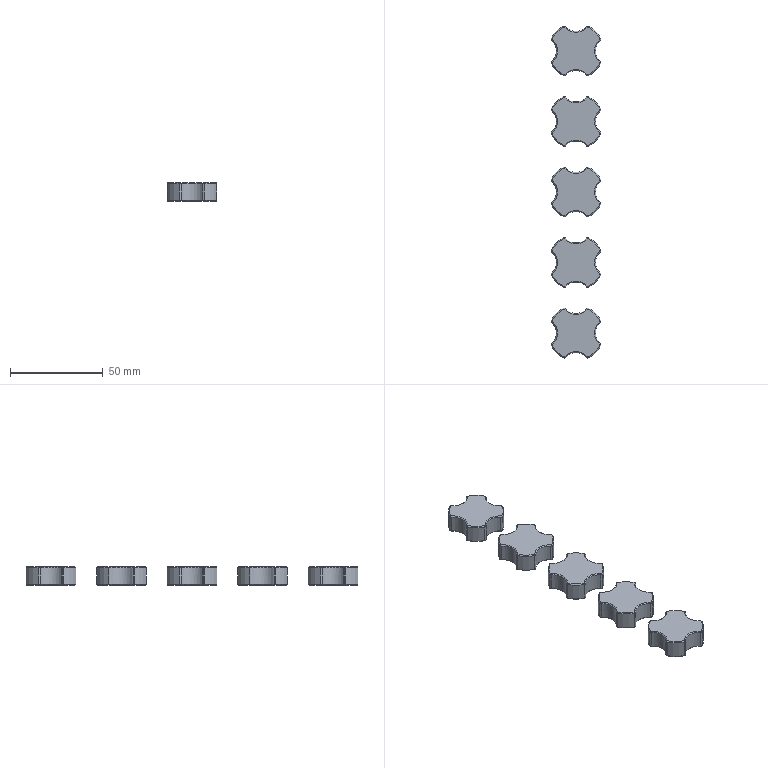NC program | NX | posted with a generic post | part box 26.875 x 178.875 x 10 mm
Lines 19 to 822 of 10509:
(ZLEVEL_PROFILE_COPY_1 , TOOL : D10)
N36 T15 M6
N38 G54
N40 G17 G0 G90 X-92.11 Y1.511 S9500 M3
N42 G43 Z30. H15
N44 Z1.5
N46 G94 G1 X-92.142 Y1.566 Z1.497 F1000.
N48 X-92.887 Y2.211 Z1.445
N50 X-93.723 Y3.322 Z1.372
N52 X-94.287 Y4.593 Z1.299
N54 X-94.55 Y5.958 Z1.226
N56 X-94.498 Y7.348 Z1.154
N58 X-94.135 Y8.689 Z1.081
N60 X-93.352 Y10.204 Z0.991
N62 X-91.921 Y12.318 Z0.858
N64 X-90.234 Y14.234 Z0.724
N66 X-88.318 Y15.921 Z0.59
N68 X-86.204 Y17.352 Z0.456
N70 X-84.689 Y18.135 Z0.367
N72 X-83.87 Y18.395 Z0.322
N74 X-83.023 Y18.538 Z0.277
N76 X-81.811 Y18.536 Z0.213
N78 X-80.5 Y18.257 Z0.143
N80 X-79.28 Y17.698 Z0.073
N82 X-78.211 Y16.887 Z0.002
N84 X-77.566 Y16.142 Z-0.049
N86 X-77.004 Y15.787 Z-0.084
N88 X-76.368 Y15.598 Z-0.119
N90 X-75.607 Y15.602 Z-0.159
N92 X-74.984 Y15.792 Z-0.193
N94 X-74.434 Y16.142 Z-0.227
N96 X-73.789 Y16.887 Z-0.279
N98 X-72.678 Y17.723 Z-0.352
N100 X-71.407 Y18.287 Z-0.424
N102 X-70.042 Y18.55 Z-0.497
N104 X-68.652 Y18.498 Z-0.57
N106 X-67.311 Y18.135 Z-0.643
N108 X-65.796 Y17.352 Z-0.732
N110 X-64.121 Y16.252 Z-0.837
N112 X-62.564 Y14.99 Z-0.942
N114 X-61.787 Y14.213 Z-1.
N116 G2 X-58.143 Y9.228 R20.1 F3500.
N118 X-59.571 Y1.815 R6.1
N120 G3 X-59.571 Y-1.815 R2.4
N122 G2 X-58.143 Y-9.228 R6.1
N124 X-66.772 Y-17.857 R20.1
N126 X-74.185 Y-16.429 R6.1
N128 G3 X-77.815 Y-16.429 R2.4
N130 G2 X-85.228 Y-17.857 R6.1
N132 X-93.857 Y-9.228 R20.1
N134 X-92.429 Y-1.815 R6.1
N136 G3 X-92.429 Y1.815 R2.4
N138 G2 X-93.857 Y9.228 R6.1
N140 X-85.228 Y17.857 R20.1
N142 X-77.815 Y16.429 R6.1
N144 G3 X-74.185 Y16.429 R2.4
N146 G2 X-66.772 Y17.857 R6.1
N148 X-61.787 Y14.213 R20.1
N150 G1 X-61.076 Y13.464 Z-1.008
N152 X-60.404 Y12.679 Z-1.016
N154 X-59.773 Y11.861 Z-1.024
N156 X-59.185 Y11.012 Z-1.032
N158 X-58.641 Y10.133 Z-1.039
N160 X-58.143 Y9.228 Z-1.047
N162 X-57.901 Y8.699 Z-1.052
N164 X-57.711 Y8.15 Z-1.056
N166 X-57.573 Y7.585 Z-1.061
N168 X-57.49 Y7.01 Z-1.065
N170 X-57.463 Y6.43 Z-1.069
N172 X-57.49 Y5.849 Z-1.074
N174 X-57.573 Y5.274 Z-1.078
N176 X-57.709 Y4.709 Z-1.083
N178 X-57.9 Y4.16 Z-1.087
N180 X-58.141 Y3.631 Z-1.092
N182 X-58.432 Y3.128 Z-1.096
N184 X-58.769 Y2.655 Z-1.1
N186 X-59.15 Y2.216 Z-1.105
N188 X-59.571 Y1.815 Z-1.109
N190 X-59.921 Y1.439 Z-1.113
N192 X-60.018 Y1.298 Z-1.115
N194 X-60.214 Y0.926 Z-1.118
N196 X-60.303 Y0.677 Z-1.12
N198 X-60.384 Y0.28 Z-1.123
N200 X-60.4 Y0. Z-1.125
N202 X-60.366 Y-0.4 Z-1.128
N204 X-60.303 Y-0.677 Z-1.13
N206 X-60.158 Y-1.051 Z-1.133
N208 X-60.018 Y-1.298 Z-1.135
N210 X-59.813 Y-1.573 Z-1.138
N212 X-59.571 Y-1.815 Z-1.141
N214 X-59.15 Y-2.216 Z-1.145
N216 X-58.769 Y-2.655 Z-1.15
N218 X-58.432 Y-3.128 Z-1.154
N220 X-58.141 Y-3.631 Z-1.158
N222 X-57.9 Y-4.16 Z-1.163
N224 X-57.709 Y-4.709 Z-1.167
N226 X-57.573 Y-5.274 Z-1.172
N228 X-57.49 Y-5.849 Z-1.176
N230 X-57.463 Y-6.43 Z-1.181
N232 X-57.49 Y-7.01 Z-1.185
N234 X-57.573 Y-7.585 Z-1.189
N236 X-57.711 Y-8.15 Z-1.194
N238 X-57.901 Y-8.699 Z-1.198
N240 X-58.143 Y-9.228 Z-1.203
N242 X-58.641 Y-10.133 Z-1.211
N244 X-59.185 Y-11.012 Z-1.218
N246 X-59.773 Y-11.861 Z-1.226
N248 X-60.404 Y-12.679 Z-1.234
N250 X-61.076 Y-13.464 Z-1.242
N252 X-61.787 Y-14.213 Z-1.25
N254 X-62.536 Y-14.924 Z-1.258
N256 X-63.321 Y-15.596 Z-1.266
N258 X-64.139 Y-16.227 Z-1.274
N260 X-64.988 Y-16.815 Z-1.282
N262 X-65.867 Y-17.359 Z-1.289
N264 X-66.772 Y-17.857 Z-1.297
N266 X-67.301 Y-18.099 Z-1.302
N268 X-67.85 Y-18.289 Z-1.306
N270 X-68.415 Y-18.427 Z-1.311
N272 X-68.99 Y-18.51 Z-1.315
N274 X-69.57 Y-18.538 Z-1.319
N276 X-70.151 Y-18.51 Z-1.324
N278 X-70.726 Y-18.427 Z-1.328
N280 X-71.291 Y-18.291 Z-1.333
N282 X-71.84 Y-18.1 Z-1.337
N284 X-72.369 Y-17.859 Z-1.342
N286 X-72.872 Y-17.568 Z-1.346
N288 X-73.345 Y-17.231 Z-1.35
N290 X-73.784 Y-16.85 Z-1.355
N292 X-74.185 Y-16.429 Z-1.359
N294 X-74.561 Y-16.079 Z-1.363
N296 X-74.702 Y-15.982 Z-1.365
N298 X-75.074 Y-15.786 Z-1.368
N300 X-75.323 Y-15.697 Z-1.37
N302 X-75.72 Y-15.616 Z-1.373
N304 X-76. Y-15.6 Z-1.375
N306 X-76.4 Y-15.634 Z-1.378
N308 X-76.677 Y-15.697 Z-1.38
N310 X-77.051 Y-15.842 Z-1.383
N312 X-77.298 Y-15.982 Z-1.385
N314 X-77.573 Y-16.187 Z-1.388
N316 X-77.815 Y-16.429 Z-1.391
N318 X-78.173 Y-16.809 Z-1.395
N320 X-78.562 Y-17.157 Z-1.399
N322 X-78.979 Y-17.47 Z-1.403
N324 X-79.422 Y-17.746 Z-1.407
N326 X-79.887 Y-17.983 Z-1.411
N328 X-80.37 Y-18.18 Z-1.415
N330 X-80.869 Y-18.335 Z-1.418
N332 X-81.378 Y-18.447 Z-1.422
N334 X-81.896 Y-18.514 Z-1.426
N336 X-82.417 Y-18.537 Z-1.43
N338 X-82.903 Y-18.519 Z-1.434
N340 X-83.386 Y-18.462 Z-1.438
N342 X-83.863 Y-18.366 Z-1.442
N344 X-84.331 Y-18.233 Z-1.445
N346 X-84.787 Y-18.063 Z-1.449
N348 X-85.228 Y-17.857 Z-1.453
N350 X-86.133 Y-17.359 Z-1.461
N352 X-87.012 Y-16.815 Z-1.468
N354 X-87.861 Y-16.227 Z-1.476
N356 X-88.679 Y-15.596 Z-1.484
N358 X-89.464 Y-14.924 Z-1.492
N360 X-90.213 Y-14.213 Z-1.5
N362 X-90.924 Y-13.464 Z-1.508
N364 X-91.596 Y-12.679 Z-1.516
N366 X-92.227 Y-11.861 Z-1.524
N368 X-92.815 Y-11.012 Z-1.532
N370 X-93.359 Y-10.133 Z-1.539
N372 X-93.857 Y-9.228 Z-1.547
N374 X-94.099 Y-8.699 Z-1.552
N376 X-94.289 Y-8.15 Z-1.556
N378 X-94.427 Y-7.585 Z-1.561
N380 X-94.51 Y-7.01 Z-1.565
N382 X-94.538 Y-6.43 Z-1.569
N384 X-94.51 Y-5.849 Z-1.574
N386 X-94.427 Y-5.274 Z-1.578
N388 X-94.291 Y-4.709 Z-1.583
N390 X-94.1 Y-4.16 Z-1.587
N392 X-93.859 Y-3.631 Z-1.592
N394 X-93.568 Y-3.128 Z-1.596
N396 X-93.231 Y-2.655 Z-1.6
N398 X-92.85 Y-2.216 Z-1.605
N400 X-92.429 Y-1.815 Z-1.609
N402 X-92.079 Y-1.439 Z-1.613
N404 X-91.982 Y-1.298 Z-1.615
N406 X-91.786 Y-0.926 Z-1.618
N408 X-91.697 Y-0.677 Z-1.62
N410 X-91.616 Y-0.28 Z-1.623
N412 X-91.6 Y0. Z-1.625
N414 X-91.634 Y0.4 Z-1.628
N416 X-91.697 Y0.677 Z-1.63
N418 X-91.842 Y1.051 Z-1.633
N420 X-91.982 Y1.298 Z-1.635
N422 X-92.187 Y1.573 Z-1.638
N424 X-92.429 Y1.815 Z-1.641
N426 X-92.85 Y2.216 Z-1.645
N428 X-93.231 Y2.655 Z-1.65
N430 X-93.568 Y3.128 Z-1.654
N432 X-93.859 Y3.631 Z-1.658
N434 X-94.1 Y4.16 Z-1.663
N436 X-94.291 Y4.709 Z-1.667
N438 X-94.427 Y5.274 Z-1.672
N440 X-94.51 Y5.849 Z-1.676
N442 X-94.538 Y6.43 Z-1.681
N444 X-94.51 Y7.01 Z-1.685
N446 X-94.427 Y7.585 Z-1.689
N448 X-94.289 Y8.15 Z-1.694
N450 X-94.099 Y8.699 Z-1.698
N452 X-93.857 Y9.228 Z-1.703
N454 X-93.359 Y10.133 Z-1.711
N456 X-92.815 Y11.012 Z-1.718
N458 X-92.227 Y11.861 Z-1.726
N460 X-91.596 Y12.679 Z-1.734
N462 X-90.924 Y13.464 Z-1.742
N464 X-90.213 Y14.213 Z-1.75
N466 X-89.464 Y14.924 Z-1.758
N468 X-88.679 Y15.596 Z-1.766
N470 X-87.861 Y16.227 Z-1.774
N472 X-87.012 Y16.815 Z-1.782
N474 X-86.133 Y17.359 Z-1.789
N476 X-85.228 Y17.857 Z-1.797
N478 X-84.787 Y18.063 Z-1.801
N480 X-84.331 Y18.233 Z-1.805
N482 X-83.863 Y18.366 Z-1.808
N484 X-83.386 Y18.462 Z-1.812
N486 X-82.903 Y18.519 Z-1.816
N488 X-82.417 Y18.537 Z-1.82
N490 X-81.896 Y18.514 Z-1.824
N492 X-81.378 Y18.447 Z-1.828
N494 X-80.869 Y18.335 Z-1.831
N496 X-80.37 Y18.18 Z-1.835
N498 X-79.887 Y17.983 Z-1.839
N500 X-79.422 Y17.746 Z-1.843
N502 X-78.979 Y17.47 Z-1.847
N504 X-78.562 Y17.157 Z-1.851
N506 X-78.173 Y16.809 Z-1.855
N508 X-77.815 Y16.429 Z-1.859
N510 X-77.442 Y16.082 Z-1.863
N512 X-77.295 Y15.979 Z-1.865
N514 X-76.921 Y15.784 Z-1.868
N516 X-76.669 Y15.695 Z-1.87
N518 X-76.271 Y15.615 Z-1.873
N520 X-75.988 Y15.6 Z-1.875
N522 X-75.591 Y15.635 Z-1.878
N524 X-75.316 Y15.7 Z-1.88
N526 X-74.944 Y15.845 Z-1.883
N528 X-74.698 Y15.984 Z-1.885
N530 X-74.426 Y16.188 Z-1.888
N532 X-74.185 Y16.429 Z-1.891
N534 X-73.784 Y16.85 Z-1.895
N536 X-73.345 Y17.231 Z-1.9
N538 X-72.872 Y17.568 Z-1.904
N540 X-72.369 Y17.859 Z-1.908
N542 X-71.84 Y18.1 Z-1.913
N544 X-71.291 Y18.291 Z-1.917
N546 X-70.726 Y18.427 Z-1.922
N548 X-70.151 Y18.51 Z-1.926
N550 X-69.57 Y18.538 Z-1.931
N552 X-68.99 Y18.51 Z-1.935
N554 X-68.415 Y18.427 Z-1.939
N556 X-67.85 Y18.289 Z-1.944
N558 X-67.301 Y18.099 Z-1.948
N560 X-66.772 Y17.857 Z-1.953
N562 X-65.867 Y17.359 Z-1.961
N564 X-64.988 Y16.815 Z-1.968
N566 X-64.139 Y16.227 Z-1.976
N568 X-63.321 Y15.596 Z-1.984
N570 X-62.536 Y14.924 Z-1.992
N572 X-61.787 Y14.213 Z-2.
N574 X-61.076 Y13.464 Z-2.008
N576 X-60.404 Y12.679 Z-2.016
N578 X-59.773 Y11.861 Z-2.024
N580 X-59.185 Y11.012 Z-2.032
N582 X-58.641 Y10.133 Z-2.039
N584 X-58.143 Y9.228 Z-2.047
N586 X-57.901 Y8.699 Z-2.052
N588 X-57.711 Y8.15 Z-2.056
N590 X-57.573 Y7.585 Z-2.061
N592 X-57.49 Y7.01 Z-2.065
N594 X-57.463 Y6.43 Z-2.069
N596 X-57.49 Y5.849 Z-2.074
N598 X-57.573 Y5.274 Z-2.078
N600 X-57.709 Y4.709 Z-2.083
N602 X-57.9 Y4.16 Z-2.087
N604 X-58.141 Y3.631 Z-2.092
N606 X-58.432 Y3.128 Z-2.096
N608 X-58.769 Y2.655 Z-2.1
N610 X-59.15 Y2.216 Z-2.105
N612 X-59.571 Y1.815 Z-2.109
N614 X-59.921 Y1.439 Z-2.113
N616 X-60.018 Y1.298 Z-2.115
N618 X-60.214 Y0.926 Z-2.118
N620 X-60.303 Y0.677 Z-2.12
N622 X-60.384 Y0.28 Z-2.123
N624 X-60.4 Y0. Z-2.125
N626 X-60.366 Y-0.4 Z-2.128
N628 X-60.303 Y-0.677 Z-2.13
N630 X-60.158 Y-1.051 Z-2.133
N632 X-60.018 Y-1.298 Z-2.135
N634 X-59.813 Y-1.573 Z-2.138
N636 X-59.571 Y-1.815 Z-2.141
N638 X-59.15 Y-2.216 Z-2.145
N640 X-58.769 Y-2.655 Z-2.15
N642 X-58.432 Y-3.128 Z-2.154
N644 X-58.141 Y-3.631 Z-2.158
N646 X-57.9 Y-4.16 Z-2.163
N648 X-57.709 Y-4.709 Z-2.167
N650 X-57.573 Y-5.274 Z-2.172
N652 X-57.49 Y-5.849 Z-2.176
N654 X-57.463 Y-6.43 Z-2.181
N656 X-57.49 Y-7.01 Z-2.185
N658 X-57.573 Y-7.585 Z-2.189
N660 X-57.711 Y-8.15 Z-2.194
N662 X-57.901 Y-8.699 Z-2.198
N664 X-58.143 Y-9.228 Z-2.203
N666 X-58.641 Y-10.133 Z-2.211
N668 X-59.185 Y-11.012 Z-2.218
N670 X-59.773 Y-11.861 Z-2.226
N672 X-60.404 Y-12.679 Z-2.234
N674 X-61.076 Y-13.464 Z-2.242
N676 X-61.787 Y-14.213 Z-2.25
N678 X-62.536 Y-14.924 Z-2.258
N680 X-63.321 Y-15.596 Z-2.266
N682 X-64.139 Y-16.227 Z-2.274
N684 X-64.988 Y-16.815 Z-2.282
N686 X-65.867 Y-17.359 Z-2.289
N688 X-66.772 Y-17.857 Z-2.297
N690 X-67.301 Y-18.099 Z-2.302
N692 X-67.85 Y-18.289 Z-2.306
N694 X-68.415 Y-18.427 Z-2.311
N696 X-68.99 Y-18.51 Z-2.315
N698 X-69.57 Y-18.538 Z-2.319
N700 X-70.151 Y-18.51 Z-2.324
N702 X-70.726 Y-18.427 Z-2.328
N704 X-71.291 Y-18.291 Z-2.333
N706 X-71.84 Y-18.1 Z-2.337
N708 X-72.369 Y-17.859 Z-2.342
N710 X-72.872 Y-17.568 Z-2.346
N712 X-73.345 Y-17.231 Z-2.35
N714 X-73.784 Y-16.85 Z-2.355
N716 X-74.185 Y-16.429 Z-2.359
N718 X-74.561 Y-16.079 Z-2.363
N720 X-74.702 Y-15.982 Z-2.365
N722 X-75.074 Y-15.786 Z-2.368
N724 X-75.323 Y-15.697 Z-2.37
N726 X-75.72 Y-15.616 Z-2.373
N728 X-76. Y-15.6 Z-2.375
N730 X-76.4 Y-15.634 Z-2.378
N732 X-76.677 Y-15.697 Z-2.38
N734 X-77.051 Y-15.842 Z-2.383
N736 X-77.298 Y-15.982 Z-2.385
N738 X-77.573 Y-16.187 Z-2.388
N740 X-77.815 Y-16.429 Z-2.391
N742 X-78.173 Y-16.809 Z-2.395
N744 X-78.562 Y-17.157 Z-2.399
N746 X-78.979 Y-17.47 Z-2.403
N748 X-79.422 Y-17.746 Z-2.407
N750 X-79.887 Y-17.983 Z-2.411
N752 X-80.37 Y-18.18 Z-2.415
N754 X-80.869 Y-18.335 Z-2.418
N756 X-81.378 Y-18.447 Z-2.422
N758 X-81.896 Y-18.514 Z-2.426
N760 X-82.417 Y-18.537 Z-2.43
N762 X-82.903 Y-18.519 Z-2.434
N764 X-83.386 Y-18.462 Z-2.438
N766 X-83.863 Y-18.366 Z-2.442
N768 X-84.331 Y-18.233 Z-2.445
N770 X-84.787 Y-18.063 Z-2.449
N772 X-85.228 Y-17.857 Z-2.453
N774 X-86.133 Y-17.359 Z-2.461
N776 X-87.012 Y-16.815 Z-2.468
N778 X-87.861 Y-16.227 Z-2.476
N780 X-88.679 Y-15.596 Z-2.484
N782 X-89.464 Y-14.924 Z-2.492
N784 X-90.213 Y-14.213 Z-2.5
N786 X-90.924 Y-13.464 Z-2.508
N788 X-91.596 Y-12.679 Z-2.516
N790 X-92.227 Y-11.861 Z-2.524
N792 X-92.815 Y-11.012 Z-2.532
N794 X-93.359 Y-10.133 Z-2.539
N796 X-93.857 Y-9.228 Z-2.547
N798 X-94.099 Y-8.699 Z-2.552
N800 X-94.289 Y-8.15 Z-2.556
N802 X-94.427 Y-7.585 Z-2.561
N804 X-94.51 Y-7.01 Z-2.565
N806 X-94.538 Y-6.43 Z-2.569
N808 X-94.51 Y-5.849 Z-2.574
N810 X-94.427 Y-5.274 Z-2.578
N812 X-94.291 Y-4.709 Z-2.583
N814 X-94.1 Y-4.16 Z-2.587
N816 X-93.859 Y-3.631 Z-2.592
N818 X-93.568 Y-3.128 Z-2.596
N820 X-93.231 Y-2.655 Z-2.6
N822 X-92.85 Y-2.216 Z-2.605
N824 X-92.429 Y-1.815 Z-2.609
N826 X-92.079 Y-1.439 Z-2.613
N828 X-91.982 Y-1.298 Z-2.615
N830 X-91.786 Y-0.926 Z-2.618
N832 X-91.697 Y-0.677 Z-2.62
N834 X-91.616 Y-0.28 Z-2.623
N836 X-91.6 Y0. Z-2.625
N838 X-91.634 Y0.4 Z-2.628
N840 X-91.697 Y0.677 Z-2.63
N842 X-91.842 Y1.051 Z-2.633
N844 X-91.982 Y1.298 Z-2.635
N846 X-92.187 Y1.573 Z-2.638
N848 X-92.429 Y1.815 Z-2.641
N850 X-92.85 Y2.216 Z-2.645
N852 X-93.231 Y2.655 Z-2.65
N854 X-93.568 Y3.128 Z-2.654
N856 X-93.859 Y3.631 Z-2.658
N858 X-94.1 Y4.16 Z-2.663
N860 X-94.291 Y4.709 Z-2.667
N862 X-94.427 Y5.274 Z-2.672
N864 X-94.51 Y5.849 Z-2.676
N866 X-94.538 Y6.43 Z-2.681
N868 X-94.51 Y7.01 Z-2.685
N870 X-94.427 Y7.585 Z-2.689
N872 X-94.289 Y8.15 Z-2.694
N874 X-94.099 Y8.699 Z-2.698
N876 X-93.857 Y9.228 Z-2.703
N878 X-93.359 Y10.133 Z-2.711
N880 X-92.815 Y11.012 Z-2.718
N882 X-92.227 Y11.861 Z-2.726
N884 X-91.596 Y12.679 Z-2.734
N886 X-90.924 Y13.464 Z-2.742
N888 X-90.213 Y14.213 Z-2.75
N890 X-89.464 Y14.924 Z-2.758
N892 X-88.679 Y15.596 Z-2.766
N894 X-87.861 Y16.227 Z-2.774
N896 X-87.012 Y16.815 Z-2.782
N898 X-86.133 Y17.359 Z-2.789
N900 X-85.228 Y17.857 Z-2.797
N902 X-84.787 Y18.063 Z-2.801
N904 X-84.331 Y18.233 Z-2.805
N906 X-83.863 Y18.366 Z-2.808
N908 X-83.386 Y18.462 Z-2.812
N910 X-82.903 Y18.519 Z-2.816
N912 X-82.417 Y18.537 Z-2.82
N914 X-81.896 Y18.514 Z-2.824
N916 X-81.378 Y18.447 Z-2.828
N918 X-80.869 Y18.335 Z-2.831
N920 X-80.37 Y18.18 Z-2.835
N922 X-79.887 Y17.983 Z-2.839
N924 X-79.422 Y17.746 Z-2.843
N926 X-78.979 Y17.47 Z-2.847
N928 X-78.562 Y17.157 Z-2.851
N930 X-78.173 Y16.809 Z-2.855
N932 X-77.815 Y16.429 Z-2.859
N934 X-77.442 Y16.082 Z-2.863
N936 X-77.295 Y15.979 Z-2.865
N938 X-76.921 Y15.784 Z-2.868
N940 X-76.669 Y15.695 Z-2.87
N942 X-76.271 Y15.615 Z-2.873
N944 X-75.988 Y15.6 Z-2.875
N946 X-75.591 Y15.635 Z-2.878
N948 X-75.316 Y15.7 Z-2.88
N950 X-74.944 Y15.845 Z-2.883
N952 X-74.698 Y15.984 Z-2.885
N954 X-74.426 Y16.188 Z-2.888
N956 X-74.185 Y16.429 Z-2.891
N958 X-73.784 Y16.85 Z-2.895
N960 X-73.345 Y17.231 Z-2.9
N962 X-72.872 Y17.568 Z-2.904
N964 X-72.369 Y17.859 Z-2.908
N966 X-71.84 Y18.1 Z-2.913
N968 X-71.291 Y18.291 Z-2.917
N970 X-70.726 Y18.427 Z-2.922
N972 X-70.151 Y18.51 Z-2.926
N974 X-69.57 Y18.538 Z-2.931
N976 X-68.99 Y18.51 Z-2.935
N978 X-68.415 Y18.427 Z-2.939
N980 X-67.85 Y18.289 Z-2.944
N982 X-67.301 Y18.099 Z-2.948
N984 X-66.772 Y17.857 Z-2.953
N986 X-65.867 Y17.359 Z-2.961
N988 X-64.988 Y16.815 Z-2.968
N990 X-64.139 Y16.227 Z-2.976
N992 X-63.321 Y15.596 Z-2.984
N994 X-62.536 Y14.924 Z-2.992
N996 X-61.787 Y14.213 Z-3.
N998 X-61.076 Y13.464 Z-3.008
N1000 X-60.404 Y12.679 Z-3.016
N1002 X-59.773 Y11.861 Z-3.024
N1004 X-59.185 Y11.012 Z-3.032
N1006 X-58.641 Y10.133 Z-3.039
N1008 X-58.143 Y9.228 Z-3.047
N1010 X-57.901 Y8.699 Z-3.052
N1012 X-57.711 Y8.15 Z-3.056
N1014 X-57.573 Y7.585 Z-3.061
N1016 X-57.49 Y7.01 Z-3.065
N1018 X-57.463 Y6.43 Z-3.069
N1020 X-57.49 Y5.849 Z-3.074
N1022 X-57.573 Y5.274 Z-3.078
N1024 X-57.709 Y4.709 Z-3.083
N1026 X-57.9 Y4.16 Z-3.087
N1028 X-58.141 Y3.631 Z-3.092
N1030 X-58.432 Y3.128 Z-3.096
N1032 X-58.769 Y2.655 Z-3.1
N1034 X-59.15 Y2.216 Z-3.105
N1036 X-59.571 Y1.815 Z-3.109
N1038 X-59.921 Y1.439 Z-3.113
N1040 X-60.018 Y1.298 Z-3.115
N1042 X-60.214 Y0.926 Z-3.118
N1044 X-60.303 Y0.677 Z-3.12
N1046 X-60.384 Y0.28 Z-3.123
N1048 X-60.4 Y0. Z-3.125
N1050 X-60.366 Y-0.4 Z-3.128
N1052 X-60.303 Y-0.677 Z-3.13
N1054 X-60.158 Y-1.051 Z-3.133
N1056 X-60.018 Y-1.298 Z-3.135
N1058 X-59.813 Y-1.573 Z-3.138
N1060 X-59.571 Y-1.815 Z-3.141
N1062 X-59.15 Y-2.216 Z-3.145
N1064 X-58.769 Y-2.655 Z-3.15
N1066 X-58.432 Y-3.128 Z-3.154
N1068 X-58.141 Y-3.631 Z-3.158
N1070 X-57.9 Y-4.16 Z-3.163
N1072 X-57.709 Y-4.709 Z-3.167
N1074 X-57.573 Y-5.274 Z-3.172
N1076 X-57.49 Y-5.849 Z-3.176
N1078 X-57.463 Y-6.43 Z-3.181
N1080 X-57.49 Y-7.01 Z-3.185
N1082 X-57.573 Y-7.585 Z-3.189
N1084 X-57.711 Y-8.15 Z-3.194
N1086 X-57.901 Y-8.699 Z-3.198
N1088 X-58.143 Y-9.228 Z-3.203
N1090 X-58.641 Y-10.133 Z-3.211
N1092 X-59.185 Y-11.012 Z-3.218
N1094 X-59.773 Y-11.861 Z-3.226
N1096 X-60.404 Y-12.679 Z-3.234
N1098 X-61.076 Y-13.464 Z-3.242
N1100 X-61.787 Y-14.213 Z-3.25
N1102 X-62.536 Y-14.924 Z-3.258
N1104 X-63.321 Y-15.596 Z-3.266
N1106 X-64.139 Y-16.227 Z-3.274
N1108 X-64.988 Y-16.815 Z-3.282
N1110 X-65.867 Y-17.359 Z-3.289
N1112 X-66.772 Y-17.857 Z-3.297
N1114 X-67.301 Y-18.099 Z-3.302
N1116 X-67.85 Y-18.289 Z-3.306
N1118 X-68.415 Y-18.427 Z-3.311
N1120 X-68.99 Y-18.51 Z-3.315
N1122 X-69.57 Y-18.538 Z-3.319
N1124 X-70.151 Y-18.51 Z-3.324
N1126 X-70.726 Y-18.427 Z-3.328
N1128 X-71.291 Y-18.291 Z-3.333
N1130 X-71.84 Y-18.1 Z-3.337
N1132 X-72.369 Y-17.859 Z-3.342
N1134 X-72.872 Y-17.568 Z-3.346
N1136 X-73.345 Y-17.231 Z-3.35
N1138 X-73.784 Y-16.85 Z-3.355
N1140 X-74.185 Y-16.429 Z-3.359
N1142 X-74.561 Y-16.079 Z-3.363
N1144 X-74.702 Y-15.982 Z-3.365
N1146 X-75.074 Y-15.786 Z-3.368
N1148 X-75.323 Y-15.697 Z-3.37
N1150 X-75.72 Y-15.616 Z-3.373
N1152 X-76. Y-15.6 Z-3.375
N1154 X-76.4 Y-15.634 Z-3.378
N1156 X-76.677 Y-15.697 Z-3.38
N1158 X-77.051 Y-15.842 Z-3.383
N1160 X-77.298 Y-15.982 Z-3.385
N1162 X-77.573 Y-16.187 Z-3.388
N1164 X-77.815 Y-16.429 Z-3.391
N1166 X-78.173 Y-16.809 Z-3.395
N1168 X-78.562 Y-17.157 Z-3.399
N1170 X-78.979 Y-17.47 Z-3.403
N1172 X-79.422 Y-17.746 Z-3.407
N1174 X-79.887 Y-17.983 Z-3.411
N1176 X-80.37 Y-18.18 Z-3.415
N1178 X-80.869 Y-18.335 Z-3.418
N1180 X-81.378 Y-18.447 Z-3.422
N1182 X-81.896 Y-18.514 Z-3.426
N1184 X-82.417 Y-18.537 Z-3.43
N1186 X-82.903 Y-18.519 Z-3.434
N1188 X-83.386 Y-18.462 Z-3.438
N1190 X-83.863 Y-18.366 Z-3.442
N1192 X-84.331 Y-18.233 Z-3.445
N1194 X-84.787 Y-18.063 Z-3.449
N1196 X-85.228 Y-17.857 Z-3.453
N1198 X-86.133 Y-17.359 Z-3.461
N1200 X-87.012 Y-16.815 Z-3.468
N1202 X-87.861 Y-16.227 Z-3.476
N1204 X-88.679 Y-15.596 Z-3.484
N1206 X-89.464 Y-14.924 Z-3.492
N1208 X-90.213 Y-14.213 Z-3.5
N1210 X-90.924 Y-13.464 Z-3.508
N1212 X-91.596 Y-12.679 Z-3.516
N1214 X-92.227 Y-11.861 Z-3.524
N1216 X-92.815 Y-11.012 Z-3.532
N1218 X-93.359 Y-10.133 Z-3.539
N1220 X-93.857 Y-9.228 Z-3.547
N1222 X-94.099 Y-8.699 Z-3.552
N1224 X-94.289 Y-8.15 Z-3.556
N1226 X-94.427 Y-7.585 Z-3.561
N1228 X-94.51 Y-7.01 Z-3.565
N1230 X-94.538 Y-6.43 Z-3.569
N1232 X-94.51 Y-5.849 Z-3.574
N1234 X-94.427 Y-5.274 Z-3.578
N1236 X-94.291 Y-4.709 Z-3.583
N1238 X-94.1 Y-4.16 Z-3.587
N1240 X-93.859 Y-3.631 Z-3.592
N1242 X-93.568 Y-3.128 Z-3.596
N1244 X-93.231 Y-2.655 Z-3.6
N1246 X-92.85 Y-2.216 Z-3.605
N1248 X-92.429 Y-1.815 Z-3.609
N1250 X-92.079 Y-1.439 Z-3.613
N1252 X-91.982 Y-1.298 Z-3.615
N1254 X-91.786 Y-0.926 Z-3.618
N1256 X-91.697 Y-0.677 Z-3.62
N1258 X-91.616 Y-0.28 Z-3.623
N1260 X-91.6 Y0. Z-3.625
N1262 X-91.634 Y0.4 Z-3.628
N1264 X-91.697 Y0.677 Z-3.63
N1266 X-91.842 Y1.051 Z-3.633
N1268 X-91.982 Y1.298 Z-3.635
N1270 X-92.187 Y1.573 Z-3.638
N1272 X-92.429 Y1.815 Z-3.641
N1274 X-92.85 Y2.216 Z-3.645
N1276 X-93.231 Y2.655 Z-3.65
N1278 X-93.568 Y3.128 Z-3.654
N1280 X-93.859 Y3.631 Z-3.658
N1282 X-94.1 Y4.16 Z-3.663
N1284 X-94.291 Y4.709 Z-3.667
N1286 X-94.427 Y5.274 Z-3.672
N1288 X-94.51 Y5.849 Z-3.676
N1290 X-94.538 Y6.43 Z-3.681
N1292 X-94.51 Y7.01 Z-3.685
N1294 X-94.427 Y7.585 Z-3.689
N1296 X-94.289 Y8.15 Z-3.694
N1298 X-94.099 Y8.699 Z-3.698
N1300 X-93.857 Y9.228 Z-3.703
N1302 X-93.359 Y10.133 Z-3.711
N1304 X-92.815 Y11.012 Z-3.718
N1306 X-92.227 Y11.861 Z-3.726
N1308 X-91.596 Y12.679 Z-3.734
N1310 X-90.924 Y13.464 Z-3.742
N1312 X-90.213 Y14.213 Z-3.75
N1314 X-89.464 Y14.924 Z-3.758
N1316 X-88.679 Y15.596 Z-3.766
N1318 X-87.861 Y16.227 Z-3.774
N1320 X-87.012 Y16.815 Z-3.782
N1322 X-86.133 Y17.359 Z-3.789
N1324 X-85.228 Y17.857 Z-3.797
N1326 X-84.787 Y18.063 Z-3.801
N1328 X-84.331 Y18.233 Z-3.805
N1330 X-83.863 Y18.366 Z-3.808
N1332 X-83.386 Y18.462 Z-3.812
N1334 X-82.903 Y18.519 Z-3.816
N1336 X-82.417 Y18.537 Z-3.82
N1338 X-81.896 Y18.514 Z-3.824
N1340 X-81.378 Y18.447 Z-3.828
N1342 X-80.869 Y18.335 Z-3.831
N1344 X-80.37 Y18.18 Z-3.835
N1346 X-79.887 Y17.983 Z-3.839
N1348 X-79.422 Y17.746 Z-3.843
N1350 X-78.979 Y17.47 Z-3.847
N1352 X-78.562 Y17.157 Z-3.851
N1354 X-78.173 Y16.809 Z-3.855
N1356 X-77.815 Y16.429 Z-3.859
N1358 X-77.442 Y16.082 Z-3.863
N1360 X-77.295 Y15.979 Z-3.865
N1362 X-76.921 Y15.784 Z-3.868
N1364 X-76.669 Y15.695 Z-3.87
N1366 X-76.271 Y15.615 Z-3.873
N1368 X-75.988 Y15.6 Z-3.875
N1370 X-75.591 Y15.635 Z-3.878
N1372 X-75.316 Y15.7 Z-3.88
N1374 X-74.944 Y15.845 Z-3.883
N1376 X-74.698 Y15.984 Z-3.885
N1378 X-74.426 Y16.188 Z-3.888
N1380 X-74.185 Y16.429 Z-3.891
N1382 X-73.784 Y16.85 Z-3.895
N1384 X-73.345 Y17.231 Z-3.9
N1386 X-72.872 Y17.568 Z-3.904
N1388 X-72.369 Y17.859 Z-3.908
N1390 X-71.84 Y18.1 Z-3.913
N1392 X-71.291 Y18.291 Z-3.917
N1394 X-70.726 Y18.427 Z-3.922
N1396 X-70.151 Y18.51 Z-3.926
N1398 X-69.57 Y18.538 Z-3.931
N1400 X-68.99 Y18.51 Z-3.935
N1402 X-68.415 Y18.427 Z-3.939
N1404 X-67.85 Y18.289 Z-3.944
N1406 X-67.301 Y18.099 Z-3.948
N1408 X-66.772 Y17.857 Z-3.953
N1410 X-65.867 Y17.359 Z-3.961
N1412 X-64.988 Y16.815 Z-3.968
N1414 X-64.139 Y16.227 Z-3.976
N1416 X-63.321 Y15.596 Z-3.984
N1418 X-62.536 Y14.924 Z-3.992
N1420 X-61.787 Y14.213 Z-4.
N1422 X-61.076 Y13.464 Z-4.008
N1424 X-60.404 Y12.679 Z-4.016
N1426 X-59.773 Y11.861 Z-4.024
N1428 X-59.185 Y11.012 Z-4.032
N1430 X-58.641 Y10.133 Z-4.039
N1432 X-58.143 Y9.228 Z-4.047
N1434 X-57.901 Y8.699 Z-4.052
N1436 X-57.711 Y8.15 Z-4.056
N1438 X-57.573 Y7.585 Z-4.061
N1440 X-57.49 Y7.01 Z-4.065
N1442 X-57.463 Y6.43 Z-4.069
N1444 X-57.49 Y5.849 Z-4.074
N1446 X-57.573 Y5.274 Z-4.078
N1448 X-57.709 Y4.709 Z-4.083
N1450 X-57.9 Y4.16 Z-4.087
N1452 X-58.141 Y3.631 Z-4.092
N1454 X-58.432 Y3.128 Z-4.096
N1456 X-58.769 Y2.655 Z-4.1
N1458 X-59.15 Y2.216 Z-4.105
N1460 X-59.571 Y1.815 Z-4.109
N1462 X-59.921 Y1.439 Z-4.113
N1464 X-60.018 Y1.298 Z-4.115
N1466 X-60.214 Y0.926 Z-4.118
N1468 X-60.303 Y0.677 Z-4.12
N1470 X-60.384 Y0.28 Z-4.123
N1472 X-60.4 Y0. Z-4.125
N1474 X-60.366 Y-0.4 Z-4.128
N1476 X-60.303 Y-0.677 Z-4.13
N1478 X-60.158 Y-1.051 Z-4.133
N1480 X-60.018 Y-1.298 Z-4.135
N1482 X-59.813 Y-1.573 Z-4.138
N1484 X-59.571 Y-1.815 Z-4.141
N1486 X-59.15 Y-2.216 Z-4.145
N1488 X-58.769 Y-2.655 Z-4.15
N1490 X-58.432 Y-3.128 Z-4.154
N1492 X-58.141 Y-3.631 Z-4.158
N1494 X-57.9 Y-4.16 Z-4.163
N1496 X-57.709 Y-4.709 Z-4.167
N1498 X-57.573 Y-5.274 Z-4.172
N1500 X-57.49 Y-5.849 Z-4.176
N1502 X-57.463 Y-6.43 Z-4.181
N1504 X-57.49 Y-7.01 Z-4.185
N1506 X-57.573 Y-7.585 Z-4.189
N1508 X-57.711 Y-8.15 Z-4.194
N1510 X-57.901 Y-8.699 Z-4.198
N1512 X-58.143 Y-9.228 Z-4.203
N1514 X-58.641 Y-10.133 Z-4.211
N1516 X-59.185 Y-11.012 Z-4.218
N1518 X-59.773 Y-11.861 Z-4.226
N1520 X-60.404 Y-12.679 Z-4.234
N1522 X-61.076 Y-13.464 Z-4.242
N1524 X-61.787 Y-14.213 Z-4.25
N1526 X-62.536 Y-14.924 Z-4.258
N1528 X-63.321 Y-15.596 Z-4.266
N1530 X-64.139 Y-16.227 Z-4.274
N1532 X-64.988 Y-16.815 Z-4.282
N1534 X-65.867 Y-17.359 Z-4.289
N1536 X-66.772 Y-17.857 Z-4.297
N1538 X-67.301 Y-18.099 Z-4.302
N1540 X-67.85 Y-18.289 Z-4.306
N1542 X-68.415 Y-18.427 Z-4.311
N1544 X-68.99 Y-18.51 Z-4.315
N1546 X-69.57 Y-18.538 Z-4.319
N1548 X-70.151 Y-18.51 Z-4.324
N1550 X-70.726 Y-18.427 Z-4.328
N1552 X-71.291 Y-18.291 Z-4.333
N1554 X-71.84 Y-18.1 Z-4.337
N1556 X-72.369 Y-17.859 Z-4.342
N1558 X-72.872 Y-17.568 Z-4.346
N1560 X-73.345 Y-17.231 Z-4.35
N1562 X-73.784 Y-16.85 Z-4.355
N1564 X-74.185 Y-16.429 Z-4.359
N1566 X-74.561 Y-16.079 Z-4.363
N1568 X-74.702 Y-15.982 Z-4.365
N1570 X-75.074 Y-15.786 Z-4.368
N1572 X-75.323 Y-15.697 Z-4.37
N1574 X-75.72 Y-15.616 Z-4.373
N1576 X-76. Y-15.6 Z-4.375
N1578 X-76.4 Y-15.634 Z-4.378
N1580 X-76.677 Y-15.697 Z-4.38
N1582 X-77.051 Y-15.842 Z-4.383
N1584 X-77.298 Y-15.982 Z-4.385
N1586 X-77.573 Y-16.187 Z-4.388
N1588 X-77.815 Y-16.429 Z-4.391
N1590 X-78.173 Y-16.809 Z-4.395
N1592 X-78.562 Y-17.157 Z-4.399
N1594 X-78.979 Y-17.47 Z-4.403
N1596 X-79.422 Y-17.746 Z-4.407
N1598 X-79.887 Y-17.983 Z-4.411
N1600 X-80.37 Y-18.18 Z-4.415
N1602 X-80.869 Y-18.335 Z-4.418
N1604 X-81.378 Y-18.447 Z-4.422
N1606 X-81.896 Y-18.514 Z-4.426
N1608 X-82.417 Y-18.537 Z-4.43
N1610 X-82.903 Y-18.519 Z-4.434
N1612 X-83.386 Y-18.462 Z-4.438
N1614 X-83.863 Y-18.366 Z-4.442
N1616 X-84.331 Y-18.233 Z-4.445
N1618 X-84.787 Y-18.063 Z-4.449
N1620 X-85.228 Y-17.857 Z-4.453
N1622 X-86.133 Y-17.359 Z-4.461
N1624 X-87.012 Y-16.815 Z-4.468
N1626 X-87.861 Y-16.227 Z-4.476
N1628 X-88.679 Y-15.596 Z-4.484
N1630 X-89.464 Y-14.924 Z-4.492
N1632 X-90.213 Y-14.213 Z-4.5
N1634 X-90.924 Y-13.464 Z-4.508
N1636 X-91.596 Y-12.679 Z-4.516